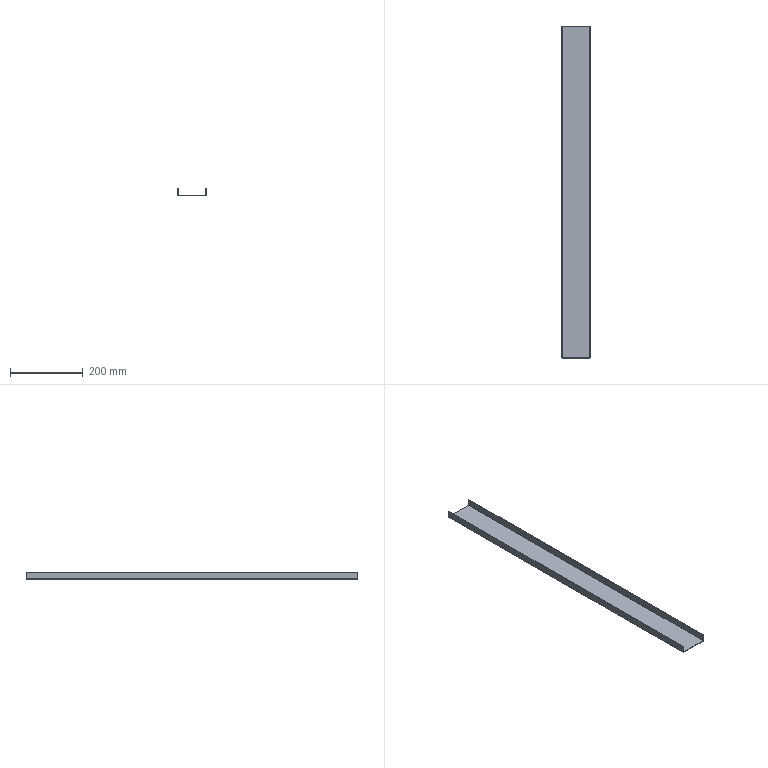Part | STEP file | 1 solid | 22 faces | box 80 x 913 x 20 mm | volume 158644 mm3 | plane 18 | cylinder 4 | commonest cylinder face diameters 1.2 x2 4.2 x2
STEP:
#1=CARTESIAN_POINT('',(0.,0.,0.));
#2=DIRECTION('',(0.,0.,1.));
#3=DIRECTION('',(1.,0.,0.));
#4=AXIS2_PLACEMENT_3D('',#1,#2,#3);
#5=CARTESIAN_POINT('',(2.1,456.5,0.));
#6=VERTEX_POINT('',#5);
#7=CARTESIAN_POINT('',(2.1,456.5,1.5));
#8=VERTEX_POINT('',#7);
#9=CARTESIAN_POINT('',(2.1,456.5,0.));
#10=DIRECTION('',(0.,0.,1.));
#11=VECTOR('',#10,1.);
#12=LINE('',#9,#11);
#13=CARTESIAN_POINT('',(2.1,456.5,0.));
#14=DIRECTION('',(0.,1.,0.));
#15=DIRECTION('',(0.,0.,1.));
#16=AXIS2_PLACEMENT_3D('',#13,#14,#15);
#17=PLANE('',#16);
#18=CARTESIAN_POINT('',(0.,0.));
#19=DIRECTION('',(1.,0.));
#20=VECTOR('',#19,1.);
#21=LINE('',#18,#20);
#22=(GEOMETRIC_REPRESENTATION_CONTEXT(2)PARAMETRIC_REPRESENTATION_CONTEXT()REPRESENTATION_CONTEXT('',''));
#23=DEFINITIONAL_REPRESENTATION('',(#21),#22);
#24=PCURVE('',#17,#23);
#25=CARTESIAN_POINT('',(1.5,456.5,2.1));
#26=DIRECTION('',(0.,1.,0.));
#27=DIRECTION('',(0.,0.,1.));
#28=AXIS2_PLACEMENT_3D('',#25,#26,#27);
#29=PLANE('',#28);
#30=CARTESIAN_POINT('',(-2.1,0.6));
#31=DIRECTION('',(1.,0.));
#32=VECTOR('',#31,1.);
#33=LINE('',#30,#32);
#34=(GEOMETRIC_REPRESENTATION_CONTEXT(2)PARAMETRIC_REPRESENTATION_CONTEXT()REPRESENTATION_CONTEXT('',''));
#35=DEFINITIONAL_REPRESENTATION('',(#33),#34);
#36=PCURVE('',#29,#35);
#37=SURFACE_CURVE('',#12,(#24,#36),.PCURVE_S1.);
#38=EDGE_CURVE('',#6,#8,#37,.T.);
#39=ORIENTED_EDGE('',*,*,#38,.F.);
#40=CARTESIAN_POINT('',(0.,456.5,2.1));
#41=VERTEX_POINT('',#40);
#42=CARTESIAN_POINT('',(2.1,456.5,2.1));
#43=DIRECTION('',(0.,-1.,0.));
#44=DIRECTION('',(0.,0.,1.));
#45=AXIS2_PLACEMENT_3D('',#42,#43,#44);
#46=CIRCLE('',#45,2.1);
#47=CARTESIAN_POINT('',(4.2,0.));
#48=CARTESIAN_POINT('',(4.2,-3.637));
#49=CARTESIAN_POINT('',(1.05,-1.819));
#50=CARTESIAN_POINT('',(-2.1,0.));
#51=CARTESIAN_POINT('',(1.05,1.819));
#52=CARTESIAN_POINT('',(4.2,3.637));
#53=CARTESIAN_POINT('',(4.2,0.));
#54=(BOUNDED_CURVE()B_SPLINE_CURVE(2,(#47,#48,#49,#50,#51,#52,#53),.UNSPECIFIED.,.T.,.F.)B_SPLINE_CURVE_WITH_KNOTS((1,2,2,2,2,1),(-2.094,0.,2.094,4.189,6.283,8.378),.UNSPECIFIED.)CURVE()GEOMETRIC_REPRESENTATION_ITEM()RATIONAL_B_SPLINE_CURVE((1.,0.5,1.,0.5,1.,0.5,1.))REPRESENTATION_ITEM(''));
#55=(GEOMETRIC_REPRESENTATION_CONTEXT(2)PARAMETRIC_REPRESENTATION_CONTEXT()REPRESENTATION_CONTEXT('',''));
#56=DEFINITIONAL_REPRESENTATION('',(#54),#55);
#57=PCURVE('',#17,#56);
#58=CARTESIAN_POINT('',(2.1,456.5,2.1));
#59=DIRECTION('',(0.,-1.,0.));
#60=DIRECTION('',(0.,0.,-1.));
#61=AXIS2_PLACEMENT_3D('',#58,#59,#60);
#62=CYLINDRICAL_SURFACE('',#61,2.1);
#63=CARTESIAN_POINT('',(3.142,0.));
#64=DIRECTION('',(1.,0.));
#65=VECTOR('',#64,1.);
#66=LINE('',#63,#65);
#67=(GEOMETRIC_REPRESENTATION_CONTEXT(2)PARAMETRIC_REPRESENTATION_CONTEXT()REPRESENTATION_CONTEXT('',''));
#68=DEFINITIONAL_REPRESENTATION('',(#66),#67);
#69=PCURVE('',#62,#68);
#70=SURFACE_CURVE('',#46,(#57,#69),.PCURVE_S1.);
#71=EDGE_CURVE('',#41,#6,#70,.T.);
#72=ORIENTED_EDGE('',*,*,#71,.F.);
#73=CARTESIAN_POINT('',(1.5,456.5,2.1));
#74=VERTEX_POINT('',#73);
#75=CARTESIAN_POINT('',(1.5,456.5,2.1));
#76=DIRECTION('',(-1.,0.,0.));
#77=VECTOR('',#76,1.);
#78=LINE('',#75,#77);
#79=CARTESIAN_POINT('',(2.1,-0.6));
#80=DIRECTION('',(0.,-1.));
#81=VECTOR('',#80,1.);
#82=LINE('',#79,#81);
#83=(GEOMETRIC_REPRESENTATION_CONTEXT(2)PARAMETRIC_REPRESENTATION_CONTEXT()REPRESENTATION_CONTEXT('',''));
#84=DEFINITIONAL_REPRESENTATION('',(#82),#83);
#85=PCURVE('',#17,#84);
#86=CARTESIAN_POINT('',(77.9,456.5,2.1));
#87=DIRECTION('',(0.,1.,0.));
#88=DIRECTION('',(1.,0.,0.));
#89=AXIS2_PLACEMENT_3D('',#86,#87,#88);
#90=PLANE('',#89);
#91=CARTESIAN_POINT('',(-76.4,0.));
#92=DIRECTION('',(-1.,0.));
#93=VECTOR('',#92,1.);
#94=LINE('',#91,#93);
#95=(GEOMETRIC_REPRESENTATION_CONTEXT(2)PARAMETRIC_REPRESENTATION_CONTEXT()REPRESENTATION_CONTEXT('',''));
#96=DEFINITIONAL_REPRESENTATION('',(#94),#95);
#97=PCURVE('',#90,#96);
#98=SURFACE_CURVE('',#78,(#85,#97),.PCURVE_S1.);
#99=EDGE_CURVE('',#74,#41,#98,.T.);
#100=ORIENTED_EDGE('',*,*,#99,.F.);
#101=CARTESIAN_POINT('',(2.1,456.5,2.1));
#102=DIRECTION('',(0.,-1.,0.));
#103=DIRECTION('',(1.,0.,0.));
#104=AXIS2_PLACEMENT_3D('',#101,#102,#103);
#105=CIRCLE('',#104,0.6);
#106=CARTESIAN_POINT('',(2.1,0.6));
#107=CARTESIAN_POINT('',(3.139,0.6));
#108=CARTESIAN_POINT('',(2.62,-0.3));
#109=CARTESIAN_POINT('',(2.1,-1.2));
#110=CARTESIAN_POINT('',(1.58,-0.3));
#111=CARTESIAN_POINT('',(1.061,0.6));
#112=CARTESIAN_POINT('',(2.1,0.6));
#113=(BOUNDED_CURVE()B_SPLINE_CURVE(2,(#106,#107,#108,#109,#110,#111,#112),.UNSPECIFIED.,.T.,.F.)B_SPLINE_CURVE_WITH_KNOTS((1,2,2,2,2,1),(-2.094,0.,2.094,4.189,6.283,8.378),.UNSPECIFIED.)CURVE()GEOMETRIC_REPRESENTATION_ITEM()RATIONAL_B_SPLINE_CURVE((1.,0.5,1.,0.5,1.,0.5,1.))REPRESENTATION_ITEM(''));
#114=(GEOMETRIC_REPRESENTATION_CONTEXT(2)PARAMETRIC_REPRESENTATION_CONTEXT()REPRESENTATION_CONTEXT('',''));
#115=DEFINITIONAL_REPRESENTATION('',(#113),#114);
#116=PCURVE('',#17,#115);
#117=CARTESIAN_POINT('',(2.1,456.5,2.1));
#118=DIRECTION('',(0.,-1.,0.));
#119=DIRECTION('',(0.,0.,-1.));
#120=AXIS2_PLACEMENT_3D('',#117,#118,#119);
#121=CYLINDRICAL_SURFACE('',#120,0.6);
#122=CARTESIAN_POINT('',(1.571,0.));
#123=DIRECTION('',(1.,0.));
#124=VECTOR('',#123,1.);
#125=LINE('',#122,#124);
#126=(GEOMETRIC_REPRESENTATION_CONTEXT(2)PARAMETRIC_REPRESENTATION_CONTEXT()REPRESENTATION_CONTEXT('',''));
#127=DEFINITIONAL_REPRESENTATION('',(#125),#126);
#128=PCURVE('',#121,#127);
#129=SURFACE_CURVE('',#105,(#116,#128),.PCURVE_S1.);
#130=EDGE_CURVE('',#74,#8,#129,.T.);
#131=ORIENTED_EDGE('',*,*,#130,.T.);
#132=EDGE_LOOP('',(#39,#72,#100,#131));
#133=FACE_BOUND('',#132,.T.);
#134=ADVANCED_FACE('',(#133),#17,.T.);
#135=CARTESIAN_POINT('',(77.9,456.5,0.));
#136=VERTEX_POINT('',#135);
#137=CARTESIAN_POINT('',(0.,456.5,0.));
#138=DIRECTION('',(1.,0.,0.));
#139=VECTOR('',#138,1.);
#140=LINE('',#137,#139);
#141=CARTESIAN_POINT('',(-2.1,-1.5));
#142=DIRECTION('',(0.,1.));
#143=VECTOR('',#142,1.);
#144=LINE('',#141,#143);
#145=(GEOMETRIC_REPRESENTATION_CONTEXT(2)PARAMETRIC_REPRESENTATION_CONTEXT()REPRESENTATION_CONTEXT('',''));
#146=DEFINITIONAL_REPRESENTATION('',(#144),#145);
#147=PCURVE('',#29,#146);
#148=CARTESIAN_POINT('',(0.,456.5,0.));
#149=DIRECTION('',(0.,0.,-1.));
#150=DIRECTION('',(-1.,0.,0.));
#151=AXIS2_PLACEMENT_3D('',#148,#149,#150);
#152=PLANE('',#151);
#153=CARTESIAN_POINT('',(0.,0.));
#154=DIRECTION('',(-1.,0.));
#155=VECTOR('',#154,1.);
#156=LINE('',#153,#155);
#157=(GEOMETRIC_REPRESENTATION_CONTEXT(2)PARAMETRIC_REPRESENTATION_CONTEXT()REPRESENTATION_CONTEXT('',''));
#158=DEFINITIONAL_REPRESENTATION('',(#156),#157);
#159=PCURVE('',#152,#158);
#160=SURFACE_CURVE('',#140,(#147,#159),.PCURVE_S1.);
#161=EDGE_CURVE('',#6,#136,#160,.T.);
#162=ORIENTED_EDGE('',*,*,#161,.F.);
#163=ORIENTED_EDGE('',*,*,#38,.T.);
#164=CARTESIAN_POINT('',(77.9,456.5,1.5));
#165=VERTEX_POINT('',#164);
#166=CARTESIAN_POINT('',(0.,456.5,1.5));
#167=DIRECTION('',(1.,0.,0.));
#168=VECTOR('',#167,1.);
#169=LINE('',#166,#168);
#170=CARTESIAN_POINT('',(-0.6,-1.5));
#171=DIRECTION('',(0.,1.));
#172=VECTOR('',#171,1.);
#173=LINE('',#170,#172);
#174=(GEOMETRIC_REPRESENTATION_CONTEXT(2)PARAMETRIC_REPRESENTATION_CONTEXT()REPRESENTATION_CONTEXT('',''));
#175=DEFINITIONAL_REPRESENTATION('',(#173),#174);
#176=PCURVE('',#29,#175);
#177=CARTESIAN_POINT('',(0.,456.5,1.5));
#178=DIRECTION('',(0.,0.,-1.));
#179=DIRECTION('',(-1.,0.,0.));
#180=AXIS2_PLACEMENT_3D('',#177,#178,#179);
#181=PLANE('',#180);
#182=CARTESIAN_POINT('',(0.,0.));
#183=DIRECTION('',(-1.,0.));
#184=VECTOR('',#183,1.);
#185=LINE('',#182,#184);
#186=(GEOMETRIC_REPRESENTATION_CONTEXT(2)PARAMETRIC_REPRESENTATION_CONTEXT()REPRESENTATION_CONTEXT('',''));
#187=DEFINITIONAL_REPRESENTATION('',(#185),#186);
#188=PCURVE('',#181,#187);
#189=SURFACE_CURVE('',#169,(#176,#188),.PCURVE_S1.);
#190=EDGE_CURVE('',#8,#165,#189,.T.);
#191=ORIENTED_EDGE('',*,*,#190,.T.);
#192=CARTESIAN_POINT('',(77.9,456.5,1.5));
#193=DIRECTION('',(0.,0.,-1.));
#194=VECTOR('',#193,1.);
#195=LINE('',#192,#194);
#196=CARTESIAN_POINT('',(-0.6,76.4));
#197=DIRECTION('',(-1.,0.));
#198=VECTOR('',#197,1.);
#199=LINE('',#196,#198);
#200=(GEOMETRIC_REPRESENTATION_CONTEXT(2)PARAMETRIC_REPRESENTATION_CONTEXT()REPRESENTATION_CONTEXT('',''));
#201=DEFINITIONAL_REPRESENTATION('',(#199),#200);
#202=PCURVE('',#29,#201);
#203=CARTESIAN_POINT('',(80.,456.5,2.1));
#204=DIRECTION('',(0.,1.,0.));
#205=DIRECTION('',(0.,0.,1.));
#206=AXIS2_PLACEMENT_3D('',#203,#204,#205);
#207=PLANE('',#206);
#208=CARTESIAN_POINT('',(-0.6,-2.1));
#209=DIRECTION('',(-1.,0.));
#210=VECTOR('',#209,1.);
#211=LINE('',#208,#210);
#212=(GEOMETRIC_REPRESENTATION_CONTEXT(2)PARAMETRIC_REPRESENTATION_CONTEXT()REPRESENTATION_CONTEXT('',''));
#213=DEFINITIONAL_REPRESENTATION('',(#211),#212);
#214=PCURVE('',#207,#213);
#215=SURFACE_CURVE('',#195,(#202,#214),.PCURVE_S1.);
#216=EDGE_CURVE('',#165,#136,#215,.T.);
#217=ORIENTED_EDGE('',*,*,#216,.T.);
#218=EDGE_LOOP('',(#162,#163,#191,#217));
#219=FACE_BOUND('',#218,.T.);
#220=ADVANCED_FACE('',(#219),#29,.T.);
#221=CARTESIAN_POINT('',(0.,-456.5,2.1));
#222=VERTEX_POINT('',#221);
#223=CARTESIAN_POINT('',(1.5,-456.5,2.1));
#224=VERTEX_POINT('',#223);
#225=CARTESIAN_POINT('',(0.,-456.5,2.1));
#226=DIRECTION('',(1.,0.,0.));
#227=VECTOR('',#226,1.);
#228=LINE('',#225,#227);
#229=CARTESIAN_POINT('',(0.,-456.5,2.1));
#230=DIRECTION('',(0.,-1.,0.));
#231=DIRECTION('',(0.,0.,-1.));
#232=AXIS2_PLACEMENT_3D('',#229,#230,#231);
#233=PLANE('',#232);
#234=CARTESIAN_POINT('',(0.,0.));
#235=DIRECTION('',(0.,1.));
#236=VECTOR('',#235,1.);
#237=LINE('',#234,#236);
#238=(GEOMETRIC_REPRESENTATION_CONTEXT(2)PARAMETRIC_REPRESENTATION_CONTEXT()REPRESENTATION_CONTEXT('',''));
#239=DEFINITIONAL_REPRESENTATION('',(#237),#238);
#240=PCURVE('',#233,#239);
#241=CARTESIAN_POINT('',(2.1,-456.5,1.5));
#242=DIRECTION('',(0.,-1.,0.));
#243=DIRECTION('',(0.,0.,-1.));
#244=AXIS2_PLACEMENT_3D('',#241,#242,#243);
#245=PLANE('',#244);
#246=CARTESIAN_POINT('',(-0.6,-2.1));
#247=DIRECTION('',(0.,1.));
#248=VECTOR('',#247,1.);
#249=LINE('',#246,#248);
#250=(GEOMETRIC_REPRESENTATION_CONTEXT(2)PARAMETRIC_REPRESENTATION_CONTEXT()REPRESENTATION_CONTEXT('',''));
#251=DEFINITIONAL_REPRESENTATION('',(#249),#250);
#252=PCURVE('',#245,#251);
#253=SURFACE_CURVE('',#228,(#240,#252),.PCURVE_S1.);
#254=EDGE_CURVE('',#222,#224,#253,.T.);
#255=ORIENTED_EDGE('',*,*,#254,.F.);
#256=CARTESIAN_POINT('',(2.1,-456.5,0.));
#257=VERTEX_POINT('',#256);
#258=CARTESIAN_POINT('',(2.1,-456.5,2.1));
#259=DIRECTION('',(0.,-1.,0.));
#260=DIRECTION('',(0.,0.,1.));
#261=AXIS2_PLACEMENT_3D('',#258,#259,#260);
#262=CIRCLE('',#261,2.1);
#263=CARTESIAN_POINT('',(0.,2.1));
#264=DIRECTION('',(-1.,0.));
#265=AXIS2_PLACEMENT_2D('',#263,#264);
#266=CIRCLE('',#265,2.1);
#267=(GEOMETRIC_REPRESENTATION_CONTEXT(2)PARAMETRIC_REPRESENTATION_CONTEXT()REPRESENTATION_CONTEXT('',''));
#268=DEFINITIONAL_REPRESENTATION('',(#266),#267);
#269=PCURVE('',#233,#268);
#270=CARTESIAN_POINT('',(3.142,913.));
#271=DIRECTION('',(1.,0.));
#272=VECTOR('',#271,1.);
#273=LINE('',#270,#272);
#274=(GEOMETRIC_REPRESENTATION_CONTEXT(2)PARAMETRIC_REPRESENTATION_CONTEXT()REPRESENTATION_CONTEXT('',''));
#275=DEFINITIONAL_REPRESENTATION('',(#273),#274);
#276=PCURVE('',#62,#275);
#277=SURFACE_CURVE('',#262,(#269,#276),.PCURVE_S1.);
#278=EDGE_CURVE('',#222,#257,#277,.T.);
#279=ORIENTED_EDGE('',*,*,#278,.T.);
#280=CARTESIAN_POINT('',(2.1,-456.5,1.5));
#281=VERTEX_POINT('',#280);
#282=CARTESIAN_POINT('',(2.1,-456.5,1.5));
#283=DIRECTION('',(0.,0.,-1.));
#284=VECTOR('',#283,1.);
#285=LINE('',#282,#284);
#286=CARTESIAN_POINT('',(0.6,2.1));
#287=DIRECTION('',(1.,0.));
#288=VECTOR('',#287,1.);
#289=LINE('',#286,#288);
#290=(GEOMETRIC_REPRESENTATION_CONTEXT(2)PARAMETRIC_REPRESENTATION_CONTEXT()REPRESENTATION_CONTEXT('',''));
#291=DEFINITIONAL_REPRESENTATION('',(#289),#290);
#292=PCURVE('',#233,#291);
#293=CARTESIAN_POINT('',(78.5,-456.5,2.1));
#294=DIRECTION('',(0.,-1.,0.));
#295=DIRECTION('',(0.,0.,-1.));
#296=AXIS2_PLACEMENT_3D('',#293,#294,#295);
#297=PLANE('',#296);
#298=CARTESIAN_POINT('',(0.6,-76.4));
#299=DIRECTION('',(1.,0.));
#300=VECTOR('',#299,1.);
#301=LINE('',#298,#300);
#302=(GEOMETRIC_REPRESENTATION_CONTEXT(2)PARAMETRIC_REPRESENTATION_CONTEXT()REPRESENTATION_CONTEXT('',''));
#303=DEFINITIONAL_REPRESENTATION('',(#301),#302);
#304=PCURVE('',#297,#303);
#305=SURFACE_CURVE('',#285,(#292,#304),.PCURVE_S1.);
#306=EDGE_CURVE('',#281,#257,#305,.T.);
#307=ORIENTED_EDGE('',*,*,#306,.F.);
#308=CARTESIAN_POINT('',(2.1,-456.5,2.1));
#309=DIRECTION('',(0.,-1.,0.));
#310=DIRECTION('',(1.,0.,0.));
#311=AXIS2_PLACEMENT_3D('',#308,#309,#310);
#312=CIRCLE('',#311,0.6);
#313=CARTESIAN_POINT('',(0.,2.1));
#314=DIRECTION('',(0.,1.));
#315=AXIS2_PLACEMENT_2D('',#313,#314);
#316=CIRCLE('',#315,0.6);
#317=(GEOMETRIC_REPRESENTATION_CONTEXT(2)PARAMETRIC_REPRESENTATION_CONTEXT()REPRESENTATION_CONTEXT('',''));
#318=DEFINITIONAL_REPRESENTATION('',(#316),#317);
#319=PCURVE('',#233,#318);
#320=CARTESIAN_POINT('',(1.571,913.));
#321=DIRECTION('',(1.,0.));
#322=VECTOR('',#321,1.);
#323=LINE('',#320,#322);
#324=(GEOMETRIC_REPRESENTATION_CONTEXT(2)PARAMETRIC_REPRESENTATION_CONTEXT()REPRESENTATION_CONTEXT('',''));
#325=DEFINITIONAL_REPRESENTATION('',(#323),#324);
#326=PCURVE('',#121,#325);
#327=SURFACE_CURVE('',#312,(#319,#326),.PCURVE_S1.);
#328=EDGE_CURVE('',#224,#281,#327,.T.);
#329=ORIENTED_EDGE('',*,*,#328,.F.);
#330=EDGE_LOOP('',(#255,#279,#307,#329));
#331=FACE_BOUND('',#330,.T.);
#332=ADVANCED_FACE('',(#331),#233,.T.);
#333=CARTESIAN_POINT('',(0.,-456.5,20.));
#334=VERTEX_POINT('',#333);
#335=CARTESIAN_POINT('',(0.,-456.5,20.));
#336=DIRECTION('',(0.,0.,-1.));
#337=VECTOR('',#336,1.);
#338=LINE('',#335,#337);
#339=CARTESIAN_POINT('',(-18.5,-2.1));
#340=DIRECTION('',(1.,0.));
#341=VECTOR('',#340,1.);
#342=LINE('',#339,#341);
#343=(GEOMETRIC_REPRESENTATION_CONTEXT(2)PARAMETRIC_REPRESENTATION_CONTEXT()REPRESENTATION_CONTEXT('',''));
#344=DEFINITIONAL_REPRESENTATION('',(#342),#343);
#345=PCURVE('',#245,#344);
#346=CARTESIAN_POINT('',(0.,456.5,20.));
#347=DIRECTION('',(-1.,0.,0.));
#348=DIRECTION('',(0.,0.,1.));
#349=AXIS2_PLACEMENT_3D('',#346,#347,#348);
#350=PLANE('',#349);
#351=CARTESIAN_POINT('',(0.,-913.));
#352=DIRECTION('',(-1.,0.));
#353=VECTOR('',#352,1.);
#354=LINE('',#351,#353);
#355=(GEOMETRIC_REPRESENTATION_CONTEXT(2)PARAMETRIC_REPRESENTATION_CONTEXT()REPRESENTATION_CONTEXT('',''));
#356=DEFINITIONAL_REPRESENTATION('',(#354),#355);
#357=PCURVE('',#350,#356);
#358=SURFACE_CURVE('',#338,(#345,#357),.PCURVE_S1.);
#359=EDGE_CURVE('',#334,#222,#358,.T.);
#360=ORIENTED_EDGE('',*,*,#359,.T.);
#361=ORIENTED_EDGE('',*,*,#254,.T.);
#362=CARTESIAN_POINT('',(1.5,-456.5,20.));
#363=VERTEX_POINT('',#362);
#364=CARTESIAN_POINT('',(1.5,-456.5,20.));
#365=DIRECTION('',(0.,0.,-1.));
#366=VECTOR('',#365,1.);
#367=LINE('',#364,#366);
#368=CARTESIAN_POINT('',(-18.5,-0.6));
#369=DIRECTION('',(1.,0.));
#370=VECTOR('',#369,1.);
#371=LINE('',#368,#370);
#372=(GEOMETRIC_REPRESENTATION_CONTEXT(2)PARAMETRIC_REPRESENTATION_CONTEXT()REPRESENTATION_CONTEXT('',''));
#373=DEFINITIONAL_REPRESENTATION('',(#371),#372);
#374=PCURVE('',#245,#373);
#375=CARTESIAN_POINT('',(1.5,456.5,20.));
#376=DIRECTION('',(-1.,0.,0.));
#377=DIRECTION('',(0.,0.,1.));
#378=AXIS2_PLACEMENT_3D('',#375,#376,#377);
#379=PLANE('',#378);
#380=CARTESIAN_POINT('',(0.,-913.));
#381=DIRECTION('',(-1.,0.));
#382=VECTOR('',#381,1.);
#383=LINE('',#380,#382);
#384=(GEOMETRIC_REPRESENTATION_CONTEXT(2)PARAMETRIC_REPRESENTATION_CONTEXT()REPRESENTATION_CONTEXT('',''));
#385=DEFINITIONAL_REPRESENTATION('',(#383),#384);
#386=PCURVE('',#379,#385);
#387=SURFACE_CURVE('',#367,(#374,#386),.PCURVE_S1.);
#388=EDGE_CURVE('',#363,#224,#387,.T.);
#389=ORIENTED_EDGE('',*,*,#388,.F.);
#390=CARTESIAN_POINT('',(1.5,-456.5,20.));
#391=DIRECTION('',(-1.,0.,0.));
#392=VECTOR('',#391,1.);
#393=LINE('',#390,#392);
#394=CARTESIAN_POINT('',(-18.5,-0.6));
#395=DIRECTION('',(0.,-1.));
#396=VECTOR('',#395,1.);
#397=LINE('',#394,#396);
#398=(GEOMETRIC_REPRESENTATION_CONTEXT(2)PARAMETRIC_REPRESENTATION_CONTEXT()REPRESENTATION_CONTEXT('',''));
#399=DEFINITIONAL_REPRESENTATION('',(#397),#398);
#400=PCURVE('',#245,#399);
#401=CARTESIAN_POINT('',(1.5,456.5,20.));
#402=DIRECTION('',(0.,0.,1.));
#403=DIRECTION('',(1.,0.,0.));
#404=AXIS2_PLACEMENT_3D('',#401,#402,#403);
#405=PLANE('',#404);
#406=CARTESIAN_POINT('',(0.,-913.));
#407=DIRECTION('',(-1.,0.));
#408=VECTOR('',#407,1.);
#409=LINE('',#406,#408);
#410=(GEOMETRIC_REPRESENTATION_CONTEXT(2)PARAMETRIC_REPRESENTATION_CONTEXT()REPRESENTATION_CONTEXT('',''));
#411=DEFINITIONAL_REPRESENTATION('',(#409),#410);
#412=PCURVE('',#405,#411);
#413=SURFACE_CURVE('',#393,(#400,#412),.PCURVE_S1.);
#414=EDGE_CURVE('',#363,#334,#413,.T.);
#415=ORIENTED_EDGE('',*,*,#414,.T.);
#416=EDGE_LOOP('',(#360,#361,#389,#415));
#417=FACE_BOUND('',#416,.T.);
#418=ADVANCED_FACE('',(#417),#245,.T.);
#419=CARTESIAN_POINT('',(80.,456.5,2.1));
#420=VERTEX_POINT('',#419);
#421=CARTESIAN_POINT('',(78.5,456.5,2.1));
#422=VERTEX_POINT('',#421);
#423=CARTESIAN_POINT('',(80.,456.5,2.1));
#424=DIRECTION('',(-1.,0.,0.));
#425=VECTOR('',#424,1.);
#426=LINE('',#423,#425);
#427=CARTESIAN_POINT('',(0.,0.));
#428=DIRECTION('',(0.,-1.));
#429=VECTOR('',#428,1.);
#430=LINE('',#427,#429);
#431=(GEOMETRIC_REPRESENTATION_CONTEXT(2)PARAMETRIC_REPRESENTATION_CONTEXT()REPRESENTATION_CONTEXT('',''));
#432=DEFINITIONAL_REPRESENTATION('',(#430),#431);
#433=PCURVE('',#207,#432);
#434=CARTESIAN_POINT('',(77.9,456.5,1.5));
#435=DIRECTION('',(0.,1.,0.));
#436=DIRECTION('',(0.,0.,1.));
#437=AXIS2_PLACEMENT_3D('',#434,#435,#436);
#438=PLANE('',#437);
#439=CARTESIAN_POINT('',(0.6,2.1));
#440=DIRECTION('',(0.,-1.));
#441=VECTOR('',#440,1.);
#442=LINE('',#439,#441);
#443=(GEOMETRIC_REPRESENTATION_CONTEXT(2)PARAMETRIC_REPRESENTATION_CONTEXT()REPRESENTATION_CONTEXT('',''));
#444=DEFINITIONAL_REPRESENTATION('',(#442),#443);
#445=PCURVE('',#438,#444);
#446=SURFACE_CURVE('',#426,(#433,#445),.PCURVE_S1.);
#447=EDGE_CURVE('',#420,#422,#446,.T.);
#448=ORIENTED_EDGE('',*,*,#447,.F.);
#449=CARTESIAN_POINT('',(77.9,456.5,2.1));
#450=DIRECTION('',(0.,-1.,0.));
#451=DIRECTION('',(0.,0.,1.));
#452=AXIS2_PLACEMENT_3D('',#449,#450,#451);
#453=CIRCLE('',#452,2.1);
#454=CARTESIAN_POINT('',(2.1,-2.1));
#455=CARTESIAN_POINT('',(2.1,-5.737));
#456=CARTESIAN_POINT('',(-1.05,-3.919));
#457=CARTESIAN_POINT('',(-4.2,-2.1));
#458=CARTESIAN_POINT('',(-1.05,-0.2813));
#459=CARTESIAN_POINT('',(2.1,1.537));
#460=CARTESIAN_POINT('',(2.1,-2.1));
#461=(BOUNDED_CURVE()B_SPLINE_CURVE(2,(#454,#455,#456,#457,#458,#459,#460),.UNSPECIFIED.,.T.,.F.)B_SPLINE_CURVE_WITH_KNOTS((1,2,2,2,2,1),(-2.094,0.,2.094,4.189,6.283,8.378),.UNSPECIFIED.)CURVE()GEOMETRIC_REPRESENTATION_ITEM()RATIONAL_B_SPLINE_CURVE((1.,0.5,1.,0.5,1.,0.5,1.))REPRESENTATION_ITEM(''));
#462=(GEOMETRIC_REPRESENTATION_CONTEXT(2)PARAMETRIC_REPRESENTATION_CONTEXT()REPRESENTATION_CONTEXT('',''));
#463=DEFINITIONAL_REPRESENTATION('',(#461),#462);
#464=PCURVE('',#207,#463);
#465=CARTESIAN_POINT('',(77.9,456.5,2.1));
#466=DIRECTION('',(0.,-1.,0.));
#467=DIRECTION('',(0.,0.,-1.));
#468=AXIS2_PLACEMENT_3D('',#465,#466,#467);
#469=CYLINDRICAL_SURFACE('',#468,2.1);
#470=CARTESIAN_POINT('',(-3.142,0.));
#471=DIRECTION('',(1.,0.));
#472=VECTOR('',#471,1.);
#473=LINE('',#470,#472);
#474=(GEOMETRIC_REPRESENTATION_CONTEXT(2)PARAMETRIC_REPRESENTATION_CONTEXT()REPRESENTATION_CONTEXT('',''));
#475=DEFINITIONAL_REPRESENTATION('',(#473),#474);
#476=PCURVE('',#469,#475);
#477=SURFACE_CURVE('',#453,(#464,#476),.PCURVE_S1.);
#478=EDGE_CURVE('',#136,#420,#477,.T.);
#479=ORIENTED_EDGE('',*,*,#478,.F.);
#480=ORIENTED_EDGE('',*,*,#216,.F.);
#481=CARTESIAN_POINT('',(77.9,456.5,2.1));
#482=DIRECTION('',(0.,-1.,0.));
#483=DIRECTION('',(1.,0.,0.));
#484=AXIS2_PLACEMENT_3D('',#481,#482,#483);
#485=CIRCLE('',#484,0.6);
#486=CARTESIAN_POINT('',(0.,-1.5));
#487=CARTESIAN_POINT('',(1.039,-1.5));
#488=CARTESIAN_POINT('',(0.5196,-2.4));
#489=CARTESIAN_POINT('',(0.,-3.3));
#490=CARTESIAN_POINT('',(-0.5196,-2.4));
#491=CARTESIAN_POINT('',(-1.039,-1.5));
#492=CARTESIAN_POINT('',(0.,-1.5));
#493=(BOUNDED_CURVE()B_SPLINE_CURVE(2,(#486,#487,#488,#489,#490,#491,#492),.UNSPECIFIED.,.T.,.F.)B_SPLINE_CURVE_WITH_KNOTS((1,2,2,2,2,1),(-2.094,0.,2.094,4.189,6.283,8.378),.UNSPECIFIED.)CURVE()GEOMETRIC_REPRESENTATION_ITEM()RATIONAL_B_SPLINE_CURVE((1.,0.5,1.,0.5,1.,0.5,1.))REPRESENTATION_ITEM(''));
#494=(GEOMETRIC_REPRESENTATION_CONTEXT(2)PARAMETRIC_REPRESENTATION_CONTEXT()REPRESENTATION_CONTEXT('',''));
#495=DEFINITIONAL_REPRESENTATION('',(#493),#494);
#496=PCURVE('',#207,#495);
#497=CARTESIAN_POINT('',(77.9,456.5,2.1));
#498=DIRECTION('',(0.,-1.,0.));
#499=DIRECTION('',(0.,0.,-1.));
#500=AXIS2_PLACEMENT_3D('',#497,#498,#499);
#501=CYLINDRICAL_SURFACE('',#500,0.6);
#502=CARTESIAN_POINT('',(-4.712,0.));
#503=DIRECTION('',(1.,0.));
#504=VECTOR('',#503,1.);
#505=LINE('',#502,#504);
#506=(GEOMETRIC_REPRESENTATION_CONTEXT(2)PARAMETRIC_REPRESENTATION_CONTEXT()REPRESENTATION_CONTEXT('',''));
#507=DEFINITIONAL_REPRESENTATION('',(#505),#506);
#508=PCURVE('',#501,#507);
#509=SURFACE_CURVE('',#485,(#496,#508),.PCURVE_S1.);
#510=EDGE_CURVE('',#165,#422,#509,.T.);
#511=ORIENTED_EDGE('',*,*,#510,.T.);
#512=EDGE_LOOP('',(#448,#479,#480,#511));
#513=FACE_BOUND('',#512,.T.);
#514=ADVANCED_FACE('',(#513),#207,.T.);
#515=CARTESIAN_POINT('',(80.,456.5,20.));
#516=VERTEX_POINT('',#515);
#517=CARTESIAN_POINT('',(80.,456.5,0.));
#518=DIRECTION('',(0.,0.,1.));
#519=VECTOR('',#518,1.);
#520=LINE('',#517,#519);
#521=CARTESIAN_POINT('',(-1.5,2.1));
#522=DIRECTION('',(1.,0.));
#523=VECTOR('',#522,1.);
#524=LINE('',#521,#523);
#525=(GEOMETRIC_REPRESENTATION_CONTEXT(2)PARAMETRIC_REPRESENTATION_CONTEXT()REPRESENTATION_CONTEXT('',''));
#526=DEFINITIONAL_REPRESENTATION('',(#524),#525);
#527=PCURVE('',#438,#526);
#528=CARTESIAN_POINT('',(80.,456.5,0.));
#529=DIRECTION('',(1.,0.,0.));
#530=DIRECTION('',(0.,0.,-1.));
#531=AXIS2_PLACEMENT_3D('',#528,#529,#530);
#532=PLANE('',#531);
#533=CARTESIAN_POINT('',(0.,0.));
#534=DIRECTION('',(-1.,0.));
#535=VECTOR('',#534,1.);
#536=LINE('',#533,#535);
#537=(GEOMETRIC_REPRESENTATION_CONTEXT(2)PARAMETRIC_REPRESENTATION_CONTEXT()REPRESENTATION_CONTEXT('',''));
#538=DEFINITIONAL_REPRESENTATION('',(#536),#537);
#539=PCURVE('',#532,#538);
#540=SURFACE_CURVE('',#520,(#527,#539),.PCURVE_S1.);
#541=EDGE_CURVE('',#420,#516,#540,.T.);
#542=ORIENTED_EDGE('',*,*,#541,.F.);
#543=ORIENTED_EDGE('',*,*,#447,.T.);
#544=CARTESIAN_POINT('',(78.5,456.5,20.));
#545=VERTEX_POINT('',#544);
#546=CARTESIAN_POINT('',(78.5,456.5,0.));
#547=DIRECTION('',(0.,0.,1.));
#548=VECTOR('',#547,1.);
#549=LINE('',#546,#548);
#550=CARTESIAN_POINT('',(-1.5,0.6));
#551=DIRECTION('',(1.,0.));
#552=VECTOR('',#551,1.);
#553=LINE('',#550,#552);
#554=(GEOMETRIC_REPRESENTATION_CONTEXT(2)PARAMETRIC_REPRESENTATION_CONTEXT()REPRESENTATION_CONTEXT('',''));
#555=DEFINITIONAL_REPRESENTATION('',(#553),#554);
#556=PCURVE('',#438,#555);
#557=CARTESIAN_POINT('',(78.5,456.5,0.));
#558=DIRECTION('',(1.,0.,0.));
#559=DIRECTION('',(0.,0.,-1.));
#560=AXIS2_PLACEMENT_3D('',#557,#558,#559);
#561=PLANE('',#560);
#562=CARTESIAN_POINT('',(0.,0.));
#563=DIRECTION('',(-1.,0.));
#564=VECTOR('',#563,1.);
#565=LINE('',#562,#564);
#566=(GEOMETRIC_REPRESENTATION_CONTEXT(2)PARAMETRIC_REPRESENTATION_CONTEXT()REPRESENTATION_CONTEXT('',''));
#567=DEFINITIONAL_REPRESENTATION('',(#565),#566);
#568=PCURVE('',#561,#567);
#569=SURFACE_CURVE('',#549,(#556,#568),.PCURVE_S1.);
#570=EDGE_CURVE('',#422,#545,#569,.T.);
#571=ORIENTED_EDGE('',*,*,#570,.T.);
#572=CARTESIAN_POINT('',(80.,456.5,20.));
#573=DIRECTION('',(-1.,0.,0.));
#574=VECTOR('',#573,1.);
#575=LINE('',#572,#574);
#576=CARTESIAN_POINT('',(18.5,2.1));
#577=DIRECTION('',(0.,-1.));
#578=VECTOR('',#577,1.);
#579=LINE('',#576,#578);
#580=(GEOMETRIC_REPRESENTATION_CONTEXT(2)PARAMETRIC_REPRESENTATION_CONTEXT()REPRESENTATION_CONTEXT('',''));
#581=DEFINITIONAL_REPRESENTATION('',(#579),#580);
#582=PCURVE('',#438,#581);
#583=CARTESIAN_POINT('',(80.,456.5,20.));
#584=DIRECTION('',(0.,0.,1.));
#585=DIRECTION('',(1.,0.,0.));
#586=AXIS2_PLACEMENT_3D('',#583,#584,#585);
#587=PLANE('',#586);
#588=CARTESIAN_POINT('',(0.,0.));
#589=DIRECTION('',(-1.,0.));
#590=VECTOR('',#589,1.);
#591=LINE('',#588,#590);
#592=(GEOMETRIC_REPRESENTATION_CONTEXT(2)PARAMETRIC_REPRESENTATION_CONTEXT()REPRESENTATION_CONTEXT('',''));
#593=DEFINITIONAL_REPRESENTATION('',(#591),#592);
#594=PCURVE('',#587,#593);
#595=SURFACE_CURVE('',#575,(#582,#594),.PCURVE_S1.);
#596=EDGE_CURVE('',#516,#545,#595,.T.);
#597=ORIENTED_EDGE('',*,*,#596,.F.);
#598=EDGE_LOOP('',(#542,#543,#571,#597));
#599=FACE_BOUND('',#598,.T.);
#600=ADVANCED_FACE('',(#599),#438,.T.);
#601=CARTESIAN_POINT('',(77.9,-456.5,0.));
#602=VERTEX_POINT('',#601);
#603=CARTESIAN_POINT('',(77.9,-456.5,1.5));
#604=VERTEX_POINT('',#603);
#605=CARTESIAN_POINT('',(77.9,-456.5,0.));
#606=DIRECTION('',(0.,0.,1.));
#607=VECTOR('',#606,1.);
#608=LINE('',#605,#607);
#609=CARTESIAN_POINT('',(77.9,-456.5,0.));
#610=DIRECTION('',(0.,-1.,0.));
#611=DIRECTION('',(0.,0.,-1.));
#612=AXIS2_PLACEMENT_3D('',#609,#610,#611);
#613=PLANE('',#612);
#614=CARTESIAN_POINT('',(0.,0.));
#615=DIRECTION('',(-1.,0.));
#616=VECTOR('',#615,1.);
#617=LINE('',#614,#616);
#618=(GEOMETRIC_REPRESENTATION_CONTEXT(2)PARAMETRIC_REPRESENTATION_CONTEXT()REPRESENTATION_CONTEXT('',''));
#619=DEFINITIONAL_REPRESENTATION('',(#617),#618);
#620=PCURVE('',#613,#619);
#621=CARTESIAN_POINT('',(2.1,-0.6));
#622=DIRECTION('',(-1.,0.));
#623=VECTOR('',#622,1.);
#624=LINE('',#621,#623);
#625=(GEOMETRIC_REPRESENTATION_CONTEXT(2)PARAMETRIC_REPRESENTATION_CONTEXT()REPRESENTATION_CONTEXT('',''));
#626=DEFINITIONAL_REPRESENTATION('',(#624),#625);
#627=PCURVE('',#297,#626);
#628=SURFACE_CURVE('',#608,(#620,#627),.PCURVE_S1.);
#629=EDGE_CURVE('',#602,#604,#628,.T.);
#630=ORIENTED_EDGE('',*,*,#629,.F.);
#631=CARTESIAN_POINT('',(80.,-456.5,2.1));
#632=VERTEX_POINT('',#631);
#633=CARTESIAN_POINT('',(77.9,-456.5,2.1));
#634=DIRECTION('',(0.,-1.,0.));
#635=DIRECTION('',(0.,0.,1.));
#636=AXIS2_PLACEMENT_3D('',#633,#634,#635);
#637=CIRCLE('',#636,2.1);
#638=CARTESIAN_POINT('',(-2.1,0.));
#639=DIRECTION('',(-1.,0.));
#640=AXIS2_PLACEMENT_2D('',#638,#639);
#641=CIRCLE('',#640,2.1);
#642=(GEOMETRIC_REPRESENTATION_CONTEXT(2)PARAMETRIC_REPRESENTATION_CONTEXT()REPRESENTATION_CONTEXT('',''));
#643=DEFINITIONAL_REPRESENTATION('',(#641),#642);
#644=PCURVE('',#613,#643);
#645=CARTESIAN_POINT('',(-3.142,913.));
#646=DIRECTION('',(1.,0.));
#647=VECTOR('',#646,1.);
#648=LINE('',#645,#647);
#649=(GEOMETRIC_REPRESENTATION_CONTEXT(2)PARAMETRIC_REPRESENTATION_CONTEXT()REPRESENTATION_CONTEXT('',''));
#650=DEFINITIONAL_REPRESENTATION('',(#648),#649);
#651=PCURVE('',#469,#650);
#652=SURFACE_CURVE('',#637,(#644,#651),.PCURVE_S1.);
#653=EDGE_CURVE('',#602,#632,#652,.T.);
#654=ORIENTED_EDGE('',*,*,#653,.T.);
#655=CARTESIAN_POINT('',(78.5,-456.5,2.1));
#656=VERTEX_POINT('',#655);
#657=CARTESIAN_POINT('',(78.5,-456.5,2.1));
#658=DIRECTION('',(1.,0.,0.));
#659=VECTOR('',#658,1.);
#660=LINE('',#657,#659);
#661=CARTESIAN_POINT('',(-2.1,0.6));
#662=DIRECTION('',(0.,1.));
#663=VECTOR('',#662,1.);
#664=LINE('',#661,#663);
#665=(GEOMETRIC_REPRESENTATION_CONTEXT(2)PARAMETRIC_REPRESENTATION_CONTEXT()REPRESENTATION_CONTEXT('',''));
#666=DEFINITIONAL_REPRESENTATION('',(#664),#665);
#667=PCURVE('',#613,#666);
#668=CARTESIAN_POINT('',(77.9,-456.5,2.1));
#669=DIRECTION('',(0.,1.,0.));
#670=DIRECTION('',(1.,0.,0.));
#671=AXIS2_PLACEMENT_3D('',#668,#669,#670);
#672=PLANE('',#671);
#673=CARTESIAN_POINT('',(0.6,0.));
#674=DIRECTION('',(1.,0.));
#675=VECTOR('',#674,1.);
#676=LINE('',#673,#675);
#677=(GEOMETRIC_REPRESENTATION_CONTEXT(2)PARAMETRIC_REPRESENTATION_CONTEXT()REPRESENTATION_CONTEXT('',''));
#678=DEFINITIONAL_REPRESENTATION('',(#676),#677);
#679=PCURVE('',#672,#678);
#680=SURFACE_CURVE('',#660,(#667,#679),.PCURVE_S1.);
#681=EDGE_CURVE('',#656,#632,#680,.T.);
#682=ORIENTED_EDGE('',*,*,#681,.F.);
#683=CARTESIAN_POINT('',(77.9,-456.5,2.1));
#684=DIRECTION('',(0.,-1.,0.));
#685=DIRECTION('',(1.,0.,0.));
#686=AXIS2_PLACEMENT_3D('',#683,#684,#685);
#687=CIRCLE('',#686,0.6);
#688=CARTESIAN_POINT('',(-2.1,0.));
#689=DIRECTION('',(0.,1.));
#690=AXIS2_PLACEMENT_2D('',#688,#689);
#691=CIRCLE('',#690,0.6);
#692=(GEOMETRIC_REPRESENTATION_CONTEXT(2)PARAMETRIC_REPRESENTATION_CONTEXT()REPRESENTATION_CONTEXT('',''));
#693=DEFINITIONAL_REPRESENTATION('',(#691),#692);
#694=PCURVE('',#613,#693);
#695=CARTESIAN_POINT('',(-4.712,913.));
#696=DIRECTION('',(1.,0.));
#697=VECTOR('',#696,1.);
#698=LINE('',#695,#697);
#699=(GEOMETRIC_REPRESENTATION_CONTEXT(2)PARAMETRIC_REPRESENTATION_CONTEXT()REPRESENTATION_CONTEXT('',''));
#700=DEFINITIONAL_REPRESENTATION('',(#698),#699);
#701=PCURVE('',#501,#700);
#702=SURFACE_CURVE('',#687,(#694,#701),.PCURVE_S1.);
#703=EDGE_CURVE('',#604,#656,#702,.T.);
#704=ORIENTED_EDGE('',*,*,#703,.F.);
#705=EDGE_LOOP('',(#630,#654,#682,#704));
#706=FACE_BOUND('',#705,.T.);
#707=ADVANCED_FACE('',(#706),#613,.T.);
#708=CARTESIAN_POINT('',(0.,-456.5,0.));
#709=DIRECTION('',(1.,0.,0.));
#710=VECTOR('',#709,1.);
#711=LINE('',#708,#710);
#712=CARTESIAN_POINT('',(2.1,-78.5));
#713=DIRECTION('',(0.,1.));
#714=VECTOR('',#713,1.);
#715=LINE('',#712,#714);
#716=(GEOMETRIC_REPRESENTATION_CONTEXT(2)PARAMETRIC_REPRESENTATION_CONTEXT()REPRESENTATION_CONTEXT('',''));
#717=DEFINITIONAL_REPRESENTATION('',(#715),#716);
#718=PCURVE('',#297,#717);
#719=CARTESIAN_POINT('',(0.,-913.));
#720=DIRECTION('',(-1.,0.));
#721=VECTOR('',#720,1.);
#722=LINE('',#719,#721);
#723=(GEOMETRIC_REPRESENTATION_CONTEXT(2)PARAMETRIC_REPRESENTATION_CONTEXT()REPRESENTATION_CONTEXT('',''));
#724=DEFINITIONAL_REPRESENTATION('',(#722),#723);
#725=PCURVE('',#152,#724);
#726=SURFACE_CURVE('',#711,(#718,#725),.PCURVE_S1.);
#727=EDGE_CURVE('',#257,#602,#726,.T.);
#728=ORIENTED_EDGE('',*,*,#727,.T.);
#729=ORIENTED_EDGE('',*,*,#629,.T.);
#730=CARTESIAN_POINT('',(0.,-456.5,1.5));
#731=DIRECTION('',(1.,0.,0.));
#732=VECTOR('',#731,1.);
#733=LINE('',#730,#732);
#734=CARTESIAN_POINT('',(0.6,-78.5));
#735=DIRECTION('',(0.,1.));
#736=VECTOR('',#735,1.);
#737=LINE('',#734,#736);
#738=(GEOMETRIC_REPRESENTATION_CONTEXT(2)PARAMETRIC_REPRESENTATION_CONTEXT()REPRESENTATION_CONTEXT('',''));
#739=DEFINITIONAL_REPRESENTATION('',(#737),#738);
#740=PCURVE('',#297,#739);
#741=CARTESIAN_POINT('',(0.,-913.));
#742=DIRECTION('',(-1.,0.));
#743=VECTOR('',#742,1.);
#744=LINE('',#741,#743);
#745=(GEOMETRIC_REPRESENTATION_CONTEXT(2)PARAMETRIC_REPRESENTATION_CONTEXT()REPRESENTATION_CONTEXT('',''));
#746=DEFINITIONAL_REPRESENTATION('',(#744),#745);
#747=PCURVE('',#181,#746);
#748=SURFACE_CURVE('',#733,(#740,#747),.PCURVE_S1.);
#749=EDGE_CURVE('',#281,#604,#748,.T.);
#750=ORIENTED_EDGE('',*,*,#749,.F.);
#751=ORIENTED_EDGE('',*,*,#306,.T.);
#752=EDGE_LOOP('',(#728,#729,#750,#751));
#753=FACE_BOUND('',#752,.T.);
#754=ADVANCED_FACE('',(#753),#297,.T.);
#755=CARTESIAN_POINT('',(78.5,-456.5,20.));
#756=VERTEX_POINT('',#755);
#757=CARTESIAN_POINT('',(78.5,-456.5,0.));
#758=DIRECTION('',(0.,0.,1.));
#759=VECTOR('',#758,1.);
#760=LINE('',#757,#759);
#761=CARTESIAN_POINT('',(0.,-913.));
#762=DIRECTION('',(-1.,0.));
#763=VECTOR('',#762,1.);
#764=LINE('',#761,#763);
#765=(GEOMETRIC_REPRESENTATION_CONTEXT(2)PARAMETRIC_REPRESENTATION_CONTEXT()REPRESENTATION_CONTEXT('',''));
#766=DEFINITIONAL_REPRESENTATION('',(#764),#765);
#767=PCURVE('',#561,#766);
#768=CARTESIAN_POINT('',(0.6,2.1));
#769=DIRECTION('',(0.,-1.));
#770=VECTOR('',#769,1.);
#771=LINE('',#768,#770);
#772=(GEOMETRIC_REPRESENTATION_CONTEXT(2)PARAMETRIC_REPRESENTATION_CONTEXT()REPRESENTATION_CONTEXT('',''));
#773=DEFINITIONAL_REPRESENTATION('',(#771),#772);
#774=PCURVE('',#672,#773);
#775=SURFACE_CURVE('',#760,(#767,#774),.PCURVE_S1.);
#776=EDGE_CURVE('',#656,#756,#775,.T.);
#777=ORIENTED_EDGE('',*,*,#776,.T.);
#778=CARTESIAN_POINT('',(78.5,456.5,20.));
#779=DIRECTION('',(0.,-1.,0.));
#780=VECTOR('',#779,1.);
#781=LINE('',#778,#780);
#782=CARTESIAN_POINT('',(-20.,0.));
#783=DIRECTION('',(0.,-1.));
#784=VECTOR('',#783,1.);
#785=LINE('',#782,#784);
#786=(GEOMETRIC_REPRESENTATION_CONTEXT(2)PARAMETRIC_REPRESENTATION_CONTEXT()REPRESENTATION_CONTEXT('',''));
#787=DEFINITIONAL_REPRESENTATION('',(#785),#786);
#788=PCURVE('',#561,#787);
#789=CARTESIAN_POINT('',(-1.5,0.));
#790=DIRECTION('',(0.,-1.));
#791=VECTOR('',#790,1.);
#792=LINE('',#789,#791);
#793=(GEOMETRIC_REPRESENTATION_CONTEXT(2)PARAMETRIC_REPRESENTATION_CONTEXT()REPRESENTATION_CONTEXT('',''));
#794=DEFINITIONAL_REPRESENTATION('',(#792),#793);
#795=PCURVE('',#587,#794);
#796=SURFACE_CURVE('',#781,(#788,#795),.PCURVE_S1.);
#797=EDGE_CURVE('',#545,#756,#796,.T.);
#798=ORIENTED_EDGE('',*,*,#797,.F.);
#799=ORIENTED_EDGE('',*,*,#570,.F.);
#800=CARTESIAN_POINT('',(78.5,456.5,2.1));
#801=DIRECTION('',(0.,-1.,0.));
#802=VECTOR('',#801,1.);
#803=LINE('',#800,#802);
#804=CARTESIAN_POINT('',(-2.1,0.));
#805=DIRECTION('',(0.,-1.));
#806=VECTOR('',#805,1.);
#807=LINE('',#804,#806);
#808=(GEOMETRIC_REPRESENTATION_CONTEXT(2)PARAMETRIC_REPRESENTATION_CONTEXT()REPRESENTATION_CONTEXT('',''));
#809=DEFINITIONAL_REPRESENTATION('',(#807),#808);
#810=PCURVE('',#561,#809);
#811=CARTESIAN_POINT('',(1.571,0.));
#812=DIRECTION('',(0.,1.));
#813=VECTOR('',#812,1.);
#814=LINE('',#811,#813);
#815=(GEOMETRIC_REPRESENTATION_CONTEXT(2)PARAMETRIC_REPRESENTATION_CONTEXT()REPRESENTATION_CONTEXT('',''));
#816=DEFINITIONAL_REPRESENTATION('',(#814),#815);
#817=PCURVE('',#501,#816);
#818=SURFACE_CURVE('',#803,(#810,#817),.PCURVE_S1.);
#819=EDGE_CURVE('',#422,#656,#818,.T.);
#820=ORIENTED_EDGE('',*,*,#819,.T.);
#821=EDGE_LOOP('',(#777,#798,#799,#820));
#822=FACE_BOUND('',#821,.T.);
#823=ADVANCED_FACE('',(#822),#561,.F.);
#824=CARTESIAN_POINT('',(80.,-456.5,20.));
#825=VERTEX_POINT('',#824);
#826=CARTESIAN_POINT('',(80.,-456.5,20.));
#827=DIRECTION('',(-1.,0.,0.));
#828=VECTOR('',#827,1.);
#829=LINE('',#826,#828);
#830=CARTESIAN_POINT('',(0.,-913.));
#831=DIRECTION('',(-1.,0.));
#832=VECTOR('',#831,1.);
#833=LINE('',#830,#832);
#834=(GEOMETRIC_REPRESENTATION_CONTEXT(2)PARAMETRIC_REPRESENTATION_CONTEXT()REPRESENTATION_CONTEXT('',''));
#835=DEFINITIONAL_REPRESENTATION('',(#833),#834);
#836=PCURVE('',#587,#835);
#837=CARTESIAN_POINT('',(2.1,-17.9));
#838=DIRECTION('',(-1.,0.));
#839=VECTOR('',#838,1.);
#840=LINE('',#837,#839);
#841=(GEOMETRIC_REPRESENTATION_CONTEXT(2)PARAMETRIC_REPRESENTATION_CONTEXT()REPRESENTATION_CONTEXT('',''));
#842=DEFINITIONAL_REPRESENTATION('',(#840),#841);
#843=PCURVE('',#672,#842);
#844=SURFACE_CURVE('',#829,(#836,#843),.PCURVE_S1.);
#845=EDGE_CURVE('',#825,#756,#844,.T.);
#846=ORIENTED_EDGE('',*,*,#845,.F.);
#847=CARTESIAN_POINT('',(80.,456.5,20.));
#848=DIRECTION('',(0.,-1.,0.));
#849=VECTOR('',#848,1.);
#850=LINE('',#847,#849);
#851=CARTESIAN_POINT('',(0.,0.));
#852=DIRECTION('',(0.,-1.));
#853=VECTOR('',#852,1.);
#854=LINE('',#851,#853);
#855=(GEOMETRIC_REPRESENTATION_CONTEXT(2)PARAMETRIC_REPRESENTATION_CONTEXT()REPRESENTATION_CONTEXT('',''));
#856=DEFINITIONAL_REPRESENTATION('',(#854),#855);
#857=PCURVE('',#587,#856);
#858=CARTESIAN_POINT('',(-20.,0.));
#859=DIRECTION('',(0.,-1.));
#860=VECTOR('',#859,1.);
#861=LINE('',#858,#860);
#862=(GEOMETRIC_REPRESENTATION_CONTEXT(2)PARAMETRIC_REPRESENTATION_CONTEXT()REPRESENTATION_CONTEXT('',''));
#863=DEFINITIONAL_REPRESENTATION('',(#861),#862);
#864=PCURVE('',#532,#863);
#865=SURFACE_CURVE('',#850,(#857,#864),.PCURVE_S1.);
#866=EDGE_CURVE('',#516,#825,#865,.T.);
#867=ORIENTED_EDGE('',*,*,#866,.F.);
#868=ORIENTED_EDGE('',*,*,#596,.T.);
#869=ORIENTED_EDGE('',*,*,#797,.T.);
#870=EDGE_LOOP('',(#846,#867,#868,#869));
#871=FACE_BOUND('',#870,.T.);
#872=ADVANCED_FACE('',(#871),#587,.T.);
#873=CARTESIAN_POINT('',(80.,-456.5,0.));
#874=DIRECTION('',(0.,0.,1.));
#875=VECTOR('',#874,1.);
#876=LINE('',#873,#875);
#877=CARTESIAN_POINT('',(0.,-913.));
#878=DIRECTION('',(-1.,0.));
#879=VECTOR('',#878,1.);
#880=LINE('',#877,#879);
#881=(GEOMETRIC_REPRESENTATION_CONTEXT(2)PARAMETRIC_REPRESENTATION_CONTEXT()REPRESENTATION_CONTEXT('',''));
#882=DEFINITIONAL_REPRESENTATION('',(#880),#881);
#883=PCURVE('',#532,#882);
#884=CARTESIAN_POINT('',(2.1,2.1));
#885=DIRECTION('',(0.,-1.));
#886=VECTOR('',#885,1.);
#887=LINE('',#884,#886);
#888=(GEOMETRIC_REPRESENTATION_CONTEXT(2)PARAMETRIC_REPRESENTATION_CONTEXT()REPRESENTATION_CONTEXT('',''));
#889=DEFINITIONAL_REPRESENTATION('',(#887),#888);
#890=PCURVE('',#672,#889);
#891=SURFACE_CURVE('',#876,(#883,#890),.PCURVE_S1.);
#892=EDGE_CURVE('',#632,#825,#891,.T.);
#893=ORIENTED_EDGE('',*,*,#892,.F.);
#894=CARTESIAN_POINT('',(80.,456.5,2.1));
#895=DIRECTION('',(0.,-1.,0.));
#896=VECTOR('',#895,1.);
#897=LINE('',#894,#896);
#898=CARTESIAN_POINT('',(-2.1,0.));
#899=DIRECTION('',(0.,-1.));
#900=VECTOR('',#899,1.);
#901=LINE('',#898,#900);
#902=(GEOMETRIC_REPRESENTATION_CONTEXT(2)PARAMETRIC_REPRESENTATION_CONTEXT()REPRESENTATION_CONTEXT('',''));
#903=DEFINITIONAL_REPRESENTATION('',(#901),#902);
#904=PCURVE('',#532,#903);
#905=CARTESIAN_POINT('',(1.571,0.));
#906=DIRECTION('',(0.,1.));
#907=VECTOR('',#906,1.);
#908=LINE('',#905,#907);
#909=(GEOMETRIC_REPRESENTATION_CONTEXT(2)PARAMETRIC_REPRESENTATION_CONTEXT()REPRESENTATION_CONTEXT('',''));
#910=DEFINITIONAL_REPRESENTATION('',(#908),#909);
#911=PCURVE('',#469,#910);
#912=SURFACE_CURVE('',#897,(#904,#911),.PCURVE_S1.);
#913=EDGE_CURVE('',#420,#632,#912,.T.);
#914=ORIENTED_EDGE('',*,*,#913,.F.);
#915=ORIENTED_EDGE('',*,*,#541,.T.);
#916=ORIENTED_EDGE('',*,*,#866,.T.);
#917=EDGE_LOOP('',(#893,#914,#915,#916));
#918=FACE_BOUND('',#917,.T.);
#919=ADVANCED_FACE('',(#918),#532,.T.);
#920=ORIENTED_EDGE('',*,*,#653,.F.);
#921=CARTESIAN_POINT('',(77.9,456.5,0.));
#922=DIRECTION('',(0.,-1.,0.));
#923=VECTOR('',#922,1.);
#924=LINE('',#921,#923);
#925=CARTESIAN_POINT('',(0.,0.));
#926=DIRECTION('',(0.,1.));
#927=VECTOR('',#926,1.);
#928=LINE('',#925,#927);
#929=(GEOMETRIC_REPRESENTATION_CONTEXT(2)PARAMETRIC_REPRESENTATION_CONTEXT()REPRESENTATION_CONTEXT('',''));
#930=DEFINITIONAL_REPRESENTATION('',(#928),#929);
#931=PCURVE('',#469,#930);
#932=CARTESIAN_POINT('',(-77.9,0.));
#933=DIRECTION('',(0.,-1.));
#934=VECTOR('',#933,1.);
#935=LINE('',#932,#934);
#936=(GEOMETRIC_REPRESENTATION_CONTEXT(2)PARAMETRIC_REPRESENTATION_CONTEXT()REPRESENTATION_CONTEXT('',''));
#937=DEFINITIONAL_REPRESENTATION('',(#935),#936);
#938=PCURVE('',#152,#937);
#939=SURFACE_CURVE('',#924,(#931,#938),.PCURVE_S1.);
#940=EDGE_CURVE('',#136,#602,#939,.T.);
#941=ORIENTED_EDGE('',*,*,#940,.F.);
#942=ORIENTED_EDGE('',*,*,#478,.T.);
#943=ORIENTED_EDGE('',*,*,#913,.T.);
#944=EDGE_LOOP('',(#920,#941,#942,#943));
#945=FACE_BOUND('',#944,.T.);
#946=ADVANCED_FACE('',(#945),#469,.T.);
#947=ORIENTED_EDGE('',*,*,#727,.F.);
#948=CARTESIAN_POINT('',(2.1,456.5,0.));
#949=DIRECTION('',(0.,-1.,0.));
#950=VECTOR('',#949,1.);
#951=LINE('',#948,#950);
#952=CARTESIAN_POINT('',(-2.1,0.));
#953=DIRECTION('',(0.,-1.));
#954=VECTOR('',#953,1.);
#955=LINE('',#952,#954);
#956=(GEOMETRIC_REPRESENTATION_CONTEXT(2)PARAMETRIC_REPRESENTATION_CONTEXT()REPRESENTATION_CONTEXT('',''));
#957=DEFINITIONAL_REPRESENTATION('',(#955),#956);
#958=PCURVE('',#152,#957);
#959=CARTESIAN_POINT('',(6.283,0.));
#960=DIRECTION('',(0.,1.));
#961=VECTOR('',#960,1.);
#962=LINE('',#959,#961);
#963=(GEOMETRIC_REPRESENTATION_CONTEXT(2)PARAMETRIC_REPRESENTATION_CONTEXT()REPRESENTATION_CONTEXT('',''));
#964=DEFINITIONAL_REPRESENTATION('',(#962),#963);
#965=PCURVE('',#62,#964);
#966=SURFACE_CURVE('',#951,(#958,#965),.PCURVE_S1.);
#967=EDGE_CURVE('',#6,#257,#966,.T.);
#968=ORIENTED_EDGE('',*,*,#967,.F.);
#969=ORIENTED_EDGE('',*,*,#161,.T.);
#970=ORIENTED_EDGE('',*,*,#940,.T.);
#971=EDGE_LOOP('',(#947,#968,#969,#970));
#972=FACE_BOUND('',#971,.T.);
#973=ADVANCED_FACE('',(#972),#152,.T.);
#974=ORIENTED_EDGE('',*,*,#278,.F.);
#975=CARTESIAN_POINT('',(0.,456.5,2.1));
#976=DIRECTION('',(0.,-1.,0.));
#977=VECTOR('',#976,1.);
#978=LINE('',#975,#977);
#979=CARTESIAN_POINT('',(4.712,0.));
#980=DIRECTION('',(0.,1.));
#981=VECTOR('',#980,1.);
#982=LINE('',#979,#981);
#983=(GEOMETRIC_REPRESENTATION_CONTEXT(2)PARAMETRIC_REPRESENTATION_CONTEXT()REPRESENTATION_CONTEXT('',''));
#984=DEFINITIONAL_REPRESENTATION('',(#982),#983);
#985=PCURVE('',#62,#984);
#986=CARTESIAN_POINT('',(-17.9,0.));
#987=DIRECTION('',(0.,-1.));
#988=VECTOR('',#987,1.);
#989=LINE('',#986,#988);
#990=(GEOMETRIC_REPRESENTATION_CONTEXT(2)PARAMETRIC_REPRESENTATION_CONTEXT()REPRESENTATION_CONTEXT('',''));
#991=DEFINITIONAL_REPRESENTATION('',(#989),#990);
#992=PCURVE('',#350,#991);
#993=SURFACE_CURVE('',#978,(#985,#992),.PCURVE_S1.);
#994=EDGE_CURVE('',#41,#222,#993,.T.);
#995=ORIENTED_EDGE('',*,*,#994,.F.);
#996=ORIENTED_EDGE('',*,*,#71,.T.);
#997=ORIENTED_EDGE('',*,*,#967,.T.);
#998=EDGE_LOOP('',(#974,#995,#996,#997));
#999=FACE_BOUND('',#998,.T.);
#1000=ADVANCED_FACE('',(#999),#62,.T.);
#1001=ORIENTED_EDGE('',*,*,#359,.F.);
#1002=CARTESIAN_POINT('',(0.,456.5,20.));
#1003=VERTEX_POINT('',#1002);
#1004=CARTESIAN_POINT('',(0.,456.5,20.));
#1005=DIRECTION('',(0.,-1.,0.));
#1006=VECTOR('',#1005,1.);
#1007=LINE('',#1004,#1006);
#1008=CARTESIAN_POINT('',(0.,0.));
#1009=DIRECTION('',(0.,-1.));
#1010=VECTOR('',#1009,1.);
#1011=LINE('',#1008,#1010);
#1012=(GEOMETRIC_REPRESENTATION_CONTEXT(2)PARAMETRIC_REPRESENTATION_CONTEXT()REPRESENTATION_CONTEXT('',''));
#1013=DEFINITIONAL_REPRESENTATION('',(#1011),#1012);
#1014=PCURVE('',#350,#1013);
#1015=CARTESIAN_POINT('',(-1.5,0.));
#1016=DIRECTION('',(0.,-1.));
#1017=VECTOR('',#1016,1.);
#1018=LINE('',#1015,#1017);
#1019=(GEOMETRIC_REPRESENTATION_CONTEXT(2)PARAMETRIC_REPRESENTATION_CONTEXT()REPRESENTATION_CONTEXT('',''));
#1020=DEFINITIONAL_REPRESENTATION('',(#1018),#1019);
#1021=PCURVE('',#405,#1020);
#1022=SURFACE_CURVE('',#1007,(#1014,#1021),.PCURVE_S1.);
#1023=EDGE_CURVE('',#1003,#334,#1022,.T.);
#1024=ORIENTED_EDGE('',*,*,#1023,.F.);
#1025=CARTESIAN_POINT('',(0.,456.5,20.));
#1026=DIRECTION('',(0.,0.,-1.));
#1027=VECTOR('',#1026,1.);
#1028=LINE('',#1025,#1027);
#1029=CARTESIAN_POINT('',(0.,0.));
#1030=DIRECTION('',(-1.,0.));
#1031=VECTOR('',#1030,1.);
#1032=LINE('',#1029,#1031);
#1033=(GEOMETRIC_REPRESENTATION_CONTEXT(2)PARAMETRIC_REPRESENTATION_CONTEXT()REPRESENTATION_CONTEXT('',''));
#1034=DEFINITIONAL_REPRESENTATION('',(#1032),#1033);
#1035=PCURVE('',#350,#1034);
#1036=CARTESIAN_POINT('',(-77.9,-17.9));
#1037=DIRECTION('',(0.,1.));
#1038=VECTOR('',#1037,1.);
#1039=LINE('',#1036,#1038);
#1040=(GEOMETRIC_REPRESENTATION_CONTEXT(2)PARAMETRIC_REPRESENTATION_CONTEXT()REPRESENTATION_CONTEXT('',''));
#1041=DEFINITIONAL_REPRESENTATION('',(#1039),#1040);
#1042=PCURVE('',#90,#1041);
#1043=SURFACE_CURVE('',#1028,(#1035,#1042),.PCURVE_S1.);
#1044=EDGE_CURVE('',#1003,#41,#1043,.T.);
#1045=ORIENTED_EDGE('',*,*,#1044,.T.);
#1046=ORIENTED_EDGE('',*,*,#994,.T.);
#1047=EDGE_LOOP('',(#1001,#1024,#1045,#1046));
#1048=FACE_BOUND('',#1047,.T.);
#1049=ADVANCED_FACE('',(#1048),#350,.T.);
#1050=ORIENTED_EDGE('',*,*,#414,.F.);
#1051=CARTESIAN_POINT('',(1.5,456.5,20.));
#1052=VERTEX_POINT('',#1051);
#1053=CARTESIAN_POINT('',(1.5,456.5,20.));
#1054=DIRECTION('',(0.,-1.,0.));
#1055=VECTOR('',#1054,1.);
#1056=LINE('',#1053,#1055);
#1057=CARTESIAN_POINT('',(0.,0.));
#1058=DIRECTION('',(0.,-1.));
#1059=VECTOR('',#1058,1.);
#1060=LINE('',#1057,#1059);
#1061=(GEOMETRIC_REPRESENTATION_CONTEXT(2)PARAMETRIC_REPRESENTATION_CONTEXT()REPRESENTATION_CONTEXT('',''));
#1062=DEFINITIONAL_REPRESENTATION('',(#1060),#1061);
#1063=PCURVE('',#405,#1062);
#1064=CARTESIAN_POINT('',(0.,0.));
#1065=DIRECTION('',(0.,-1.));
#1066=VECTOR('',#1065,1.);
#1067=LINE('',#1064,#1066);
#1068=(GEOMETRIC_REPRESENTATION_CONTEXT(2)PARAMETRIC_REPRESENTATION_CONTEXT()REPRESENTATION_CONTEXT('',''));
#1069=DEFINITIONAL_REPRESENTATION('',(#1067),#1068);
#1070=PCURVE('',#379,#1069);
#1071=SURFACE_CURVE('',#1056,(#1063,#1070),.PCURVE_S1.);
#1072=EDGE_CURVE('',#1052,#363,#1071,.T.);
#1073=ORIENTED_EDGE('',*,*,#1072,.F.);
#1074=CARTESIAN_POINT('',(1.5,456.5,20.));
#1075=DIRECTION('',(-1.,0.,0.));
#1076=VECTOR('',#1075,1.);
#1077=LINE('',#1074,#1076);
#1078=CARTESIAN_POINT('',(0.,0.));
#1079=DIRECTION('',(-1.,0.));
#1080=VECTOR('',#1079,1.);
#1081=LINE('',#1078,#1080);
#1082=(GEOMETRIC_REPRESENTATION_CONTEXT(2)PARAMETRIC_REPRESENTATION_CONTEXT()REPRESENTATION_CONTEXT('',''));
#1083=DEFINITIONAL_REPRESENTATION('',(#1081),#1082);
#1084=PCURVE('',#405,#1083);
#1085=CARTESIAN_POINT('',(-76.4,-17.9));
#1086=DIRECTION('',(-1.,0.));
#1087=VECTOR('',#1086,1.);
#1088=LINE('',#1085,#1087);
#1089=(GEOMETRIC_REPRESENTATION_CONTEXT(2)PARAMETRIC_REPRESENTATION_CONTEXT()REPRESENTATION_CONTEXT('',''));
#1090=DEFINITIONAL_REPRESENTATION('',(#1088),#1089);
#1091=PCURVE('',#90,#1090);
#1092=SURFACE_CURVE('',#1077,(#1084,#1091),.PCURVE_S1.);
#1093=EDGE_CURVE('',#1052,#1003,#1092,.T.);
#1094=ORIENTED_EDGE('',*,*,#1093,.T.);
#1095=ORIENTED_EDGE('',*,*,#1023,.T.);
#1096=EDGE_LOOP('',(#1050,#1073,#1094,#1095));
#1097=FACE_BOUND('',#1096,.T.);
#1098=ADVANCED_FACE('',(#1097),#405,.T.);
#1099=ORIENTED_EDGE('',*,*,#388,.T.);
#1100=CARTESIAN_POINT('',(1.5,456.5,2.1));
#1101=DIRECTION('',(0.,-1.,0.));
#1102=VECTOR('',#1101,1.);
#1103=LINE('',#1100,#1102);
#1104=CARTESIAN_POINT('',(-17.9,0.));
#1105=DIRECTION('',(0.,-1.));
#1106=VECTOR('',#1105,1.);
#1107=LINE('',#1104,#1106);
#1108=(GEOMETRIC_REPRESENTATION_CONTEXT(2)PARAMETRIC_REPRESENTATION_CONTEXT()REPRESENTATION_CONTEXT('',''));
#1109=DEFINITIONAL_REPRESENTATION('',(#1107),#1108);
#1110=PCURVE('',#379,#1109);
#1111=CARTESIAN_POINT('',(4.712,0.));
#1112=DIRECTION('',(0.,1.));
#1113=VECTOR('',#1112,1.);
#1114=LINE('',#1111,#1113);
#1115=(GEOMETRIC_REPRESENTATION_CONTEXT(2)PARAMETRIC_REPRESENTATION_CONTEXT()REPRESENTATION_CONTEXT('',''));
#1116=DEFINITIONAL_REPRESENTATION('',(#1114),#1115);
#1117=PCURVE('',#121,#1116);
#1118=SURFACE_CURVE('',#1103,(#1110,#1117),.PCURVE_S1.);
#1119=EDGE_CURVE('',#74,#224,#1118,.T.);
#1120=ORIENTED_EDGE('',*,*,#1119,.F.);
#1121=CARTESIAN_POINT('',(1.5,456.5,20.));
#1122=DIRECTION('',(0.,0.,-1.));
#1123=VECTOR('',#1122,1.);
#1124=LINE('',#1121,#1123);
#1125=CARTESIAN_POINT('',(0.,0.));
#1126=DIRECTION('',(-1.,0.));
#1127=VECTOR('',#1126,1.);
#1128=LINE('',#1125,#1127);
#1129=(GEOMETRIC_REPRESENTATION_CONTEXT(2)PARAMETRIC_REPRESENTATION_CONTEXT()REPRESENTATION_CONTEXT('',''));
#1130=DEFINITIONAL_REPRESENTATION('',(#1128),#1129);
#1131=PCURVE('',#379,#1130);
#1132=CARTESIAN_POINT('',(-76.4,-17.9));
#1133=DIRECTION('',(0.,1.));
#1134=VECTOR('',#1133,1.);
#1135=LINE('',#1132,#1134);
#1136=(GEOMETRIC_REPRESENTATION_CONTEXT(2)PARAMETRIC_REPRESENTATION_CONTEXT()REPRESENTATION_CONTEXT('',''));
#1137=DEFINITIONAL_REPRESENTATION('',(#1135),#1136);
#1138=PCURVE('',#90,#1137);
#1139=SURFACE_CURVE('',#1124,(#1131,#1138),.PCURVE_S1.);
#1140=EDGE_CURVE('',#1052,#74,#1139,.T.);
#1141=ORIENTED_EDGE('',*,*,#1140,.F.);
#1142=ORIENTED_EDGE('',*,*,#1072,.T.);
#1143=EDGE_LOOP('',(#1099,#1120,#1141,#1142));
#1144=FACE_BOUND('',#1143,.T.);
#1145=ADVANCED_FACE('',(#1144),#379,.F.);
#1146=ORIENTED_EDGE('',*,*,#1119,.F.);
#1147=ORIENTED_EDGE('',*,*,#130,.T.);
#1148=CARTESIAN_POINT('',(2.1,456.5,1.5));
#1149=DIRECTION('',(0.,-1.,0.));
#1150=VECTOR('',#1149,1.);
#1151=LINE('',#1148,#1150);
#1152=CARTESIAN_POINT('',(6.283,0.));
#1153=DIRECTION('',(0.,1.));
#1154=VECTOR('',#1153,1.);
#1155=LINE('',#1152,#1154);
#1156=(GEOMETRIC_REPRESENTATION_CONTEXT(2)PARAMETRIC_REPRESENTATION_CONTEXT()REPRESENTATION_CONTEXT('',''));
#1157=DEFINITIONAL_REPRESENTATION('',(#1155),#1156);
#1158=PCURVE('',#121,#1157);
#1159=CARTESIAN_POINT('',(-2.1,0.));
#1160=DIRECTION('',(0.,-1.));
#1161=VECTOR('',#1160,1.);
#1162=LINE('',#1159,#1161);
#1163=(GEOMETRIC_REPRESENTATION_CONTEXT(2)PARAMETRIC_REPRESENTATION_CONTEXT()REPRESENTATION_CONTEXT('',''));
#1164=DEFINITIONAL_REPRESENTATION('',(#1162),#1163);
#1165=PCURVE('',#181,#1164);
#1166=SURFACE_CURVE('',#1151,(#1158,#1165),.PCURVE_S1.);
#1167=EDGE_CURVE('',#8,#281,#1166,.T.);
#1168=ORIENTED_EDGE('',*,*,#1167,.T.);
#1169=ORIENTED_EDGE('',*,*,#328,.F.);
#1170=EDGE_LOOP('',(#1146,#1147,#1168,#1169));
#1171=FACE_BOUND('',#1170,.F.);
#1172=ADVANCED_FACE('',(#1171),#121,.F.);
#1173=ORIENTED_EDGE('',*,*,#749,.T.);
#1174=CARTESIAN_POINT('',(77.9,456.5,1.5));
#1175=DIRECTION('',(0.,-1.,0.));
#1176=VECTOR('',#1175,1.);
#1177=LINE('',#1174,#1176);
#1178=CARTESIAN_POINT('',(-77.9,0.));
#1179=DIRECTION('',(0.,-1.));
#1180=VECTOR('',#1179,1.);
#1181=LINE('',#1178,#1180);
#1182=(GEOMETRIC_REPRESENTATION_CONTEXT(2)PARAMETRIC_REPRESENTATION_CONTEXT()REPRESENTATION_CONTEXT('',''));
#1183=DEFINITIONAL_REPRESENTATION('',(#1181),#1182);
#1184=PCURVE('',#181,#1183);
#1185=CARTESIAN_POINT('',(0.,0.));
#1186=DIRECTION('',(0.,1.));
#1187=VECTOR('',#1186,1.);
#1188=LINE('',#1185,#1187);
#1189=(GEOMETRIC_REPRESENTATION_CONTEXT(2)PARAMETRIC_REPRESENTATION_CONTEXT()REPRESENTATION_CONTEXT('',''));
#1190=DEFINITIONAL_REPRESENTATION('',(#1188),#1189);
#1191=PCURVE('',#501,#1190);
#1192=SURFACE_CURVE('',#1177,(#1184,#1191),.PCURVE_S1.);
#1193=EDGE_CURVE('',#165,#604,#1192,.T.);
#1194=ORIENTED_EDGE('',*,*,#1193,.F.);
#1195=ORIENTED_EDGE('',*,*,#190,.F.);
#1196=ORIENTED_EDGE('',*,*,#1167,.T.);
#1197=EDGE_LOOP('',(#1173,#1194,#1195,#1196));
#1198=FACE_BOUND('',#1197,.T.);
#1199=ADVANCED_FACE('',(#1198),#181,.F.);
#1200=ORIENTED_EDGE('',*,*,#1193,.F.);
#1201=ORIENTED_EDGE('',*,*,#510,.T.);
#1202=ORIENTED_EDGE('',*,*,#819,.T.);
#1203=ORIENTED_EDGE('',*,*,#703,.F.);
#1204=EDGE_LOOP('',(#1200,#1201,#1202,#1203));
#1205=FACE_BOUND('',#1204,.F.);
#1206=ADVANCED_FACE('',(#1205),#501,.F.);
#1207=ORIENTED_EDGE('',*,*,#1140,.T.);
#1208=ORIENTED_EDGE('',*,*,#99,.T.);
#1209=ORIENTED_EDGE('',*,*,#1044,.F.);
#1210=ORIENTED_EDGE('',*,*,#1093,.F.);
#1211=EDGE_LOOP('',(#1207,#1208,#1209,#1210));
#1212=FACE_BOUND('',#1211,.T.);
#1213=ADVANCED_FACE('',(#1212),#90,.T.);
#1214=ORIENTED_EDGE('',*,*,#776,.F.);
#1215=ORIENTED_EDGE('',*,*,#681,.T.);
#1216=ORIENTED_EDGE('',*,*,#892,.T.);
#1217=ORIENTED_EDGE('',*,*,#845,.T.);
#1218=EDGE_LOOP('',(#1214,#1215,#1216,#1217));
#1219=FACE_BOUND('',#1218,.T.);
#1220=ADVANCED_FACE('',(#1219),#672,.F.);
#1221=CLOSED_SHELL('',(#134,#220,#332,#418,#514,#600,#707,#754,#823,#872,#919,#946,#973,#1000,#1049,#1098,#1145,#1172,#1199,#1206,#1213,#1220));
#1222=MANIFOLD_SOLID_BREP('',#1221);
#1223=(LENGTH_UNIT()NAMED_UNIT(*)SI_UNIT(.MILLI.,.METRE.));
#1224=UNCERTAINTY_MEASURE_WITH_UNIT(LENGTH_MEASURE(0.0000001),#1223,'','');
#1225=(NAMED_UNIT(*)PLANE_ANGLE_UNIT()SI_UNIT($,.RADIAN.));
#1226=(NAMED_UNIT(*)SI_UNIT($,.STERADIAN.)SOLID_ANGLE_UNIT());
#1227=(GEOMETRIC_REPRESENTATION_CONTEXT(3)GLOBAL_UNCERTAINTY_ASSIGNED_CONTEXT((#1224))GLOBAL_UNIT_ASSIGNED_CONTEXT((#1223,#1225,#1226))REPRESENTATION_CONTEXT('',''));
#1228=ADVANCED_BREP_SHAPE_REPRESENTATION('',(#4,#1222),#1227);